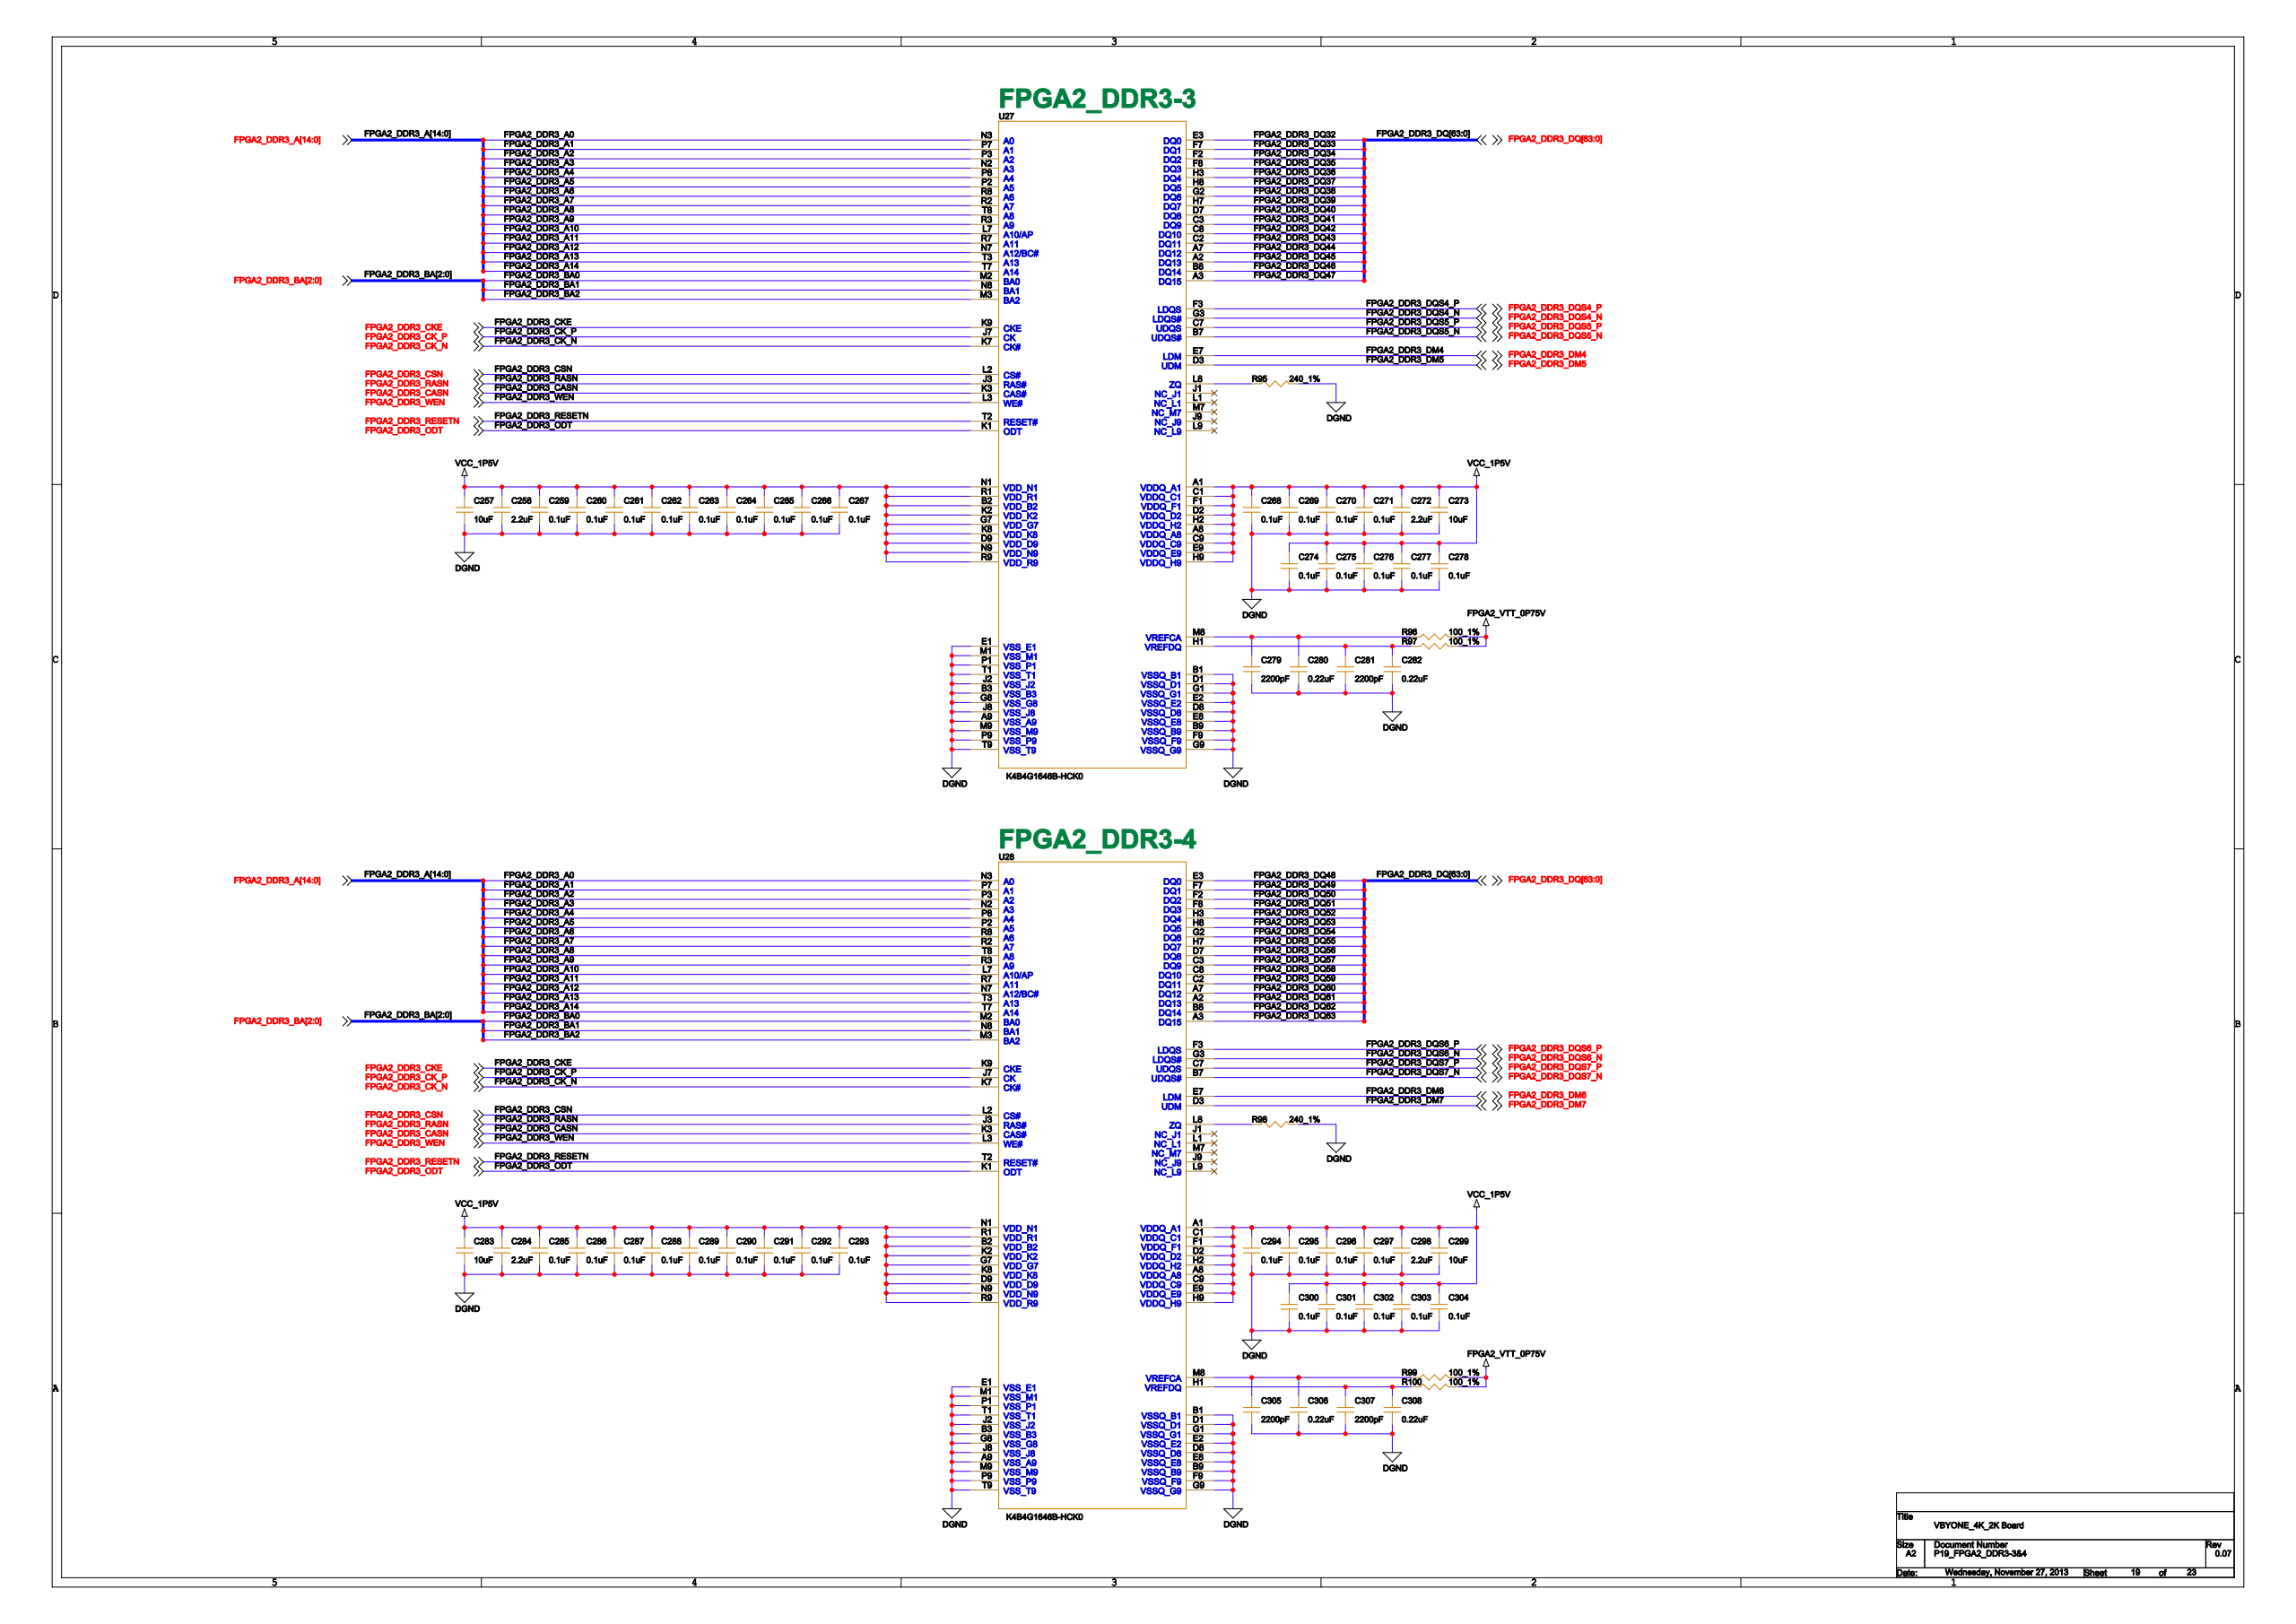Circuit board | Cadence Allegro | 1712 parts | 1495 nets | one sheet of the schematic
Parts on this sheet (reference | value | footprint):
C257 | 10uF | CRC2012RZAS
C258 | 2.2uF | CRC1608RZAS
C259 | 0.1uF | CRC1005RZAS
C260 | 0.1uF | CRC1005RZAS
C261 | 0.1uF | CRC1005RZAS
C262 | 0.1uF | CRC1005RZAS
C263 | 0.1uF | CRC1005RZAS
C264 | 0.1uF | CRC1005RZAS
C265 | 0.1uF | CRC1005RZAS
C266 | 0.1uF | CRC1005RZAS
C267 | 0.1uF | CRC1005RZAS
C268 | 0.1uF | CRC1005RZAS
C269 | 0.1uF | CRC1005RZAS
C270 | 0.1uF | CRC1005RZAS
C271 | 0.1uF | CRC1005RZAS
C272 | 2.2uF | CRC1608RZAS
C273 | 10uF | CRC2012RZAS
C274 | 0.1uF | CRC1005RZAS
C275 | 0.1uF | CRC1005RZAS
C276 | 0.1uF | CRC1005RZAS
C277 | 0.1uF | CRC1005RZAS
C278 | 0.1uF | CRC1005RZAS
C279 | 2200pF | CRC1608RZAS
C280 | 0.22uF | CRC1608RZAS
C281 | 2200pF | CRC1608RZAS
C282 | 0.22uF | CRC1608RZAS
C283 | 10uF | CRC2012RZAS
C284 | 2.2uF | CRC1608RZAS
C285 | 0.1uF | CRC1005RZAS
C286 | 0.1uF | CRC1005RZAS
C287 | 0.1uF | CRC1005RZAS
C288 | 0.1uF | CRC1005RZAS
C289 | 0.1uF | CRC1005RZAS
C290 | 0.1uF | CRC1005RZAS
C291 | 0.1uF | CRC1005RZAS
C292 | 0.1uF | CRC1005RZAS
C293 | 0.1uF | CRC1005RZAS
C294 | 0.1uF | CRC1005RZAS
C295 | 0.1uF | CRC1005RZAS
C296 | 0.1uF | CRC1005RZAS
C297 | 0.1uF | CRC1005RZAS
C298 | 2.2uF | CRC1608RZAS
C299 | 10uF | CRC2012RZAS
C300 | 0.1uF | CRC1005RZAS
C301 | 0.1uF | CRC1005RZAS
C302 | 0.1uF | CRC1005RZAS
C303 | 0.1uF | CRC1005RZAS
C304 | 0.1uF | CRC1005RZAS
C305 | 2200pF | CRC1608RZAS
C306 | 0.22uF | CRC1608RZAS
C307 | 2200pF | CRC1608RZAS
C308 | 0.22uF | CRC1608RZAS
R95 | 240_1% | CRC1608RZAS
R96 | 100_1% | CRC1005RZAS
R97 | 100_1% | CRC1005RZAS
R98 | 240_1% | CRC1608RZAS
R99 | 100_1% | CRC1005RZAS
R100 | 100_1% | CRC1005RZAS
U27 | K4B4G1646B-HCK0 | BGA096RFDS
U28 | K4B4G1646B-HCK0 | BGA096RFDS
Nets of these parts (net: part-pin ...):
DGND: C257-2 C258-2 C259-2 C260-2 C261-2 C262-2 C263-2 C264-2 C265-2 C266-2 C267-2 C268-2 C269-2 C270-2 C271-2 C272-2 C273-2 C274-2 C275-2 C276-2 C277-2 C278-2 C279-2 C280-2 C281-2 C282-2 C283-2 C284-2 C285-2 C286-2 C287-2 C288-2 C289-2 C290-2 C291-2 C292-2 C293-2 C294-2 C295-2 C296-2 C297-2 C298-2 C299-2 C300-2 C301-2 C302-2 C303-2 C304-2 C305-2 C306-2 C307-2 C308-2 R95-2 R98-2 U27-A9 U27-B1 U27-B3 U27-B9 U27-D1 U27-D8 U27-E1 U27-E2 U27-E8 U27-F9 U27-G1 U27-G8 U27-G9 U27-J2 U27-J8 U27-M1 U27-M9 U27-P1 U27-P9 U27-T1 U27-T9 U28-A9 U28-B1 U28-B3 U28-B9 U28-D1 U28-D8 U28-E1 U28-E2 U28-E8 U28-F9 U28-G1 U28-G8 U28-G9 U28-J2 U28-J8 U28-M1 U28-M9 U28-P1 U28-P9 U28-T1 U28-T9
VCC_1P5V: C257-1 C258-1 C259-1 C260-1 C261-1 C262-1 C263-1 C264-1 C265-1 C266-1 C267-1 C268-1 C269-1 C270-1 C271-1 C272-1 C273-1 C274-1 C275-1 C276-1 C277-1 C278-1 C283-1 C284-1 C285-1 C286-1 C287-1 C288-1 C289-1 C290-1 C291-1 C292-1 C293-1 C294-1 C295-1 C296-1 C297-1 C298-1 C299-1 C300-1 C301-1 C302-1 C303-1 C304-1 U27-A1 U27-A8 U27-B2 U27-C1 U27-C9 U27-D2 U27-D9 U27-E9 U27-F1 U27-G7 U27-H2 U27-H9 U27-K2 U27-K8 U27-N1 U27-N9 U27-R1 U27-R9 U28-A1 U28-A8 U28-B2 U28-C1 U28-C9 U28-D2 U28-D9 U28-E9 U28-F1 U28-G7 U28-H2 U28-H9 U28-K2 U28-K8 U28-N1 U28-N9 U28-R1 U28-R9
FPGA2_VTT_0P75V: R96-2 R97-2 R99-2 R100-2
N15850120: C279-1 C280-1 R96-1 U27-M8
N15850128: C281-1 C282-1 R97-1 U27-H1
N15852230: C305-1 C306-1 R99-1 U28-M8
N15852258: C307-1 C308-1 R100-1 U28-H1
FPGA2_DDR3_CKE: U27-K9 U28-K9
FPGA2_DDR3_RESETN: U27-T2 U28-T2
FPGA2_DDR3_ODT: U27-K1 U28-K1
FPGA2_DDR3_CSN: U27-L2 U28-L2
FPGA2_DDR3_A0: U27-N3 U28-N3
FPGA2_DDR3_A1: U27-P7 U28-P7
FPGA2_DDR3_A2: U27-P3 U28-P3
FPGA2_DDR3_A3: U27-N2 U28-N2
FPGA2_DDR3_A4: U27-P8 U28-P8
FPGA2_DDR3_A5: U27-P2 U28-P2
FPGA2_DDR3_A6: U27-R8 U28-R8
FPGA2_DDR3_A7: U27-R2 U28-R2
FPGA2_DDR3_A8: U27-T8 U28-T8
FPGA2_DDR3_A9: U27-R3 U28-R3
FPGA2_DDR3_A10: U27-L7 U28-L7
FPGA2_DDR3_A11: U27-R7 U28-R7
FPGA2_DDR3_A12: U27-N7 U28-N7
FPGA2_DDR3_A13: U27-T3 U28-T3
FPGA2_DDR3_BA0: U27-M2 U28-M2
FPGA2_DDR3_BA1: U27-N8 U28-N8
FPGA2_DDR3_BA2: U27-M3 U28-M3
FPGA2_DDR3_A14: U27-T7 U28-T7
FPGA2_DDR3_RASN: U27-J3 U28-J3
FPGA2_DDR3_CASN: U27-K3 U28-K3
FPGA2_DDR3_WEN: U27-L3 U28-L3
FPGA2_DDR3_CK_P: U27-J7 U28-J7
FPGA2_DDR3_CK_N: U27-K7 U28-K7
N15851930: R95-1 U27-L8
N15853510: R98-1 U28-L8
FPGA2_DDR3_DQ36: U27-H3
FPGA2_DDR3_DQ59: U28-C2
FPGA2_DDR3_DQ58: U28-C8
FPGA2_DDR3_DQ32: U27-E3
FPGA2_DDR3_DQ34: U27-F2
FPGA2_DDR3_DQ33: U27-F7
FPGA2_DDR3_DQ35: U27-F8
FPGA2_DDR3_DM7: U28-D3
FPGA2_DDR3_DQS7_N: U28-B7
FPGA2_DDR3_DQ57: U28-C3
FPGA2_DDR3_DQ56: U28-D7
FPGA2_DDR3_DQ63: U28-A3
FPGA2_DDR3_DM4: U27-E7
FPGA2_DDR3_DQS4_N: U27-G3
FPGA2_DDR3_DQS4_P: U27-F3
FPGA2_DDR3_DQ39: U27-H7
FPGA2_DDR3_DQ50: U28-F2
FPGA2_DDR3_DQS7_P: U28-C7
FPGA2_DDR3_DQ61: U28-A2
FPGA2_DDR3_DQ62: U28-B8
FPGA2_DDR3_DQ38: U27-G2
FPGA2_DDR3_DQ37: U27-H8
FPGA2_DDR3_DQ47: U27-A3
FPGA2_DDR3_DQ49: U28-F7
FPGA2_DDR3_DQ55: U28-H7
FPGA2_DDR3_DQ60: U28-A7
FPGA2_DDR3_DQS5_N: U27-B7
FPGA2_DDR3_DQS5_P: U27-C7
FPGA2_DDR3_DQ46: U27-B8
FPGA2_DDR3_DQ45: U27-A2
FPGA2_DDR3_DQ48: U28-E3
FPGA2_DDR3_DM6: U28-E7
FPGA2_DDR3_DQ52: U28-H3
FPGA2_DDR3_DQ51: U28-F8
FPGA2_DDR3_DQS6_N: U28-G3
FPGA2_DDR3_DQ40: U27-D7
FPGA2_DDR3_DM5: U27-D3
FPGA2_DDR3_DQ42: U27-C8
FPGA2_DDR3_DQ41: U27-C3
FPGA2_DDR3_DQ44: U27-A7
FPGA2_DDR3_DQ43: U27-C2
FPGA2_DDR3_DQ54: U28-G2
FPGA2_DDR3_DQ53: U28-H8
FPGA2_DDR3_DQS6_P: U28-F3